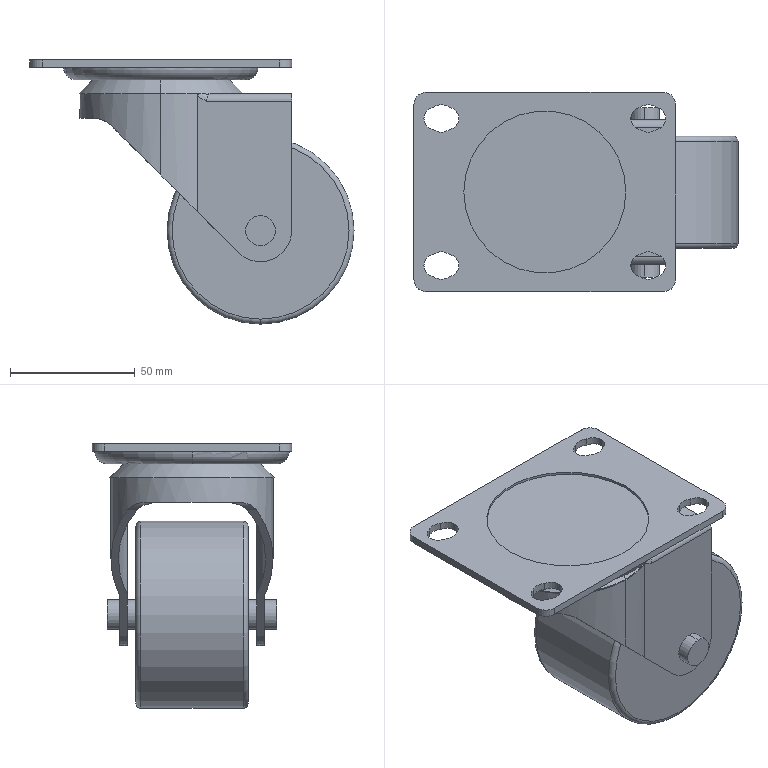Part | SolidWorks | features ICE 12, Fillet 4, Revolution 2, Extrusion 1 | 1 solid | 83 faces | box 130 x 80 x 106 mm | volume 293823 mm3 | cylinder 50 | plane 23 | torus 6 | cone 2 | spline 2 | commonest cylinder face diameters 9 x12 11 x8 12 x8 65 x5 6 x4 10 x4